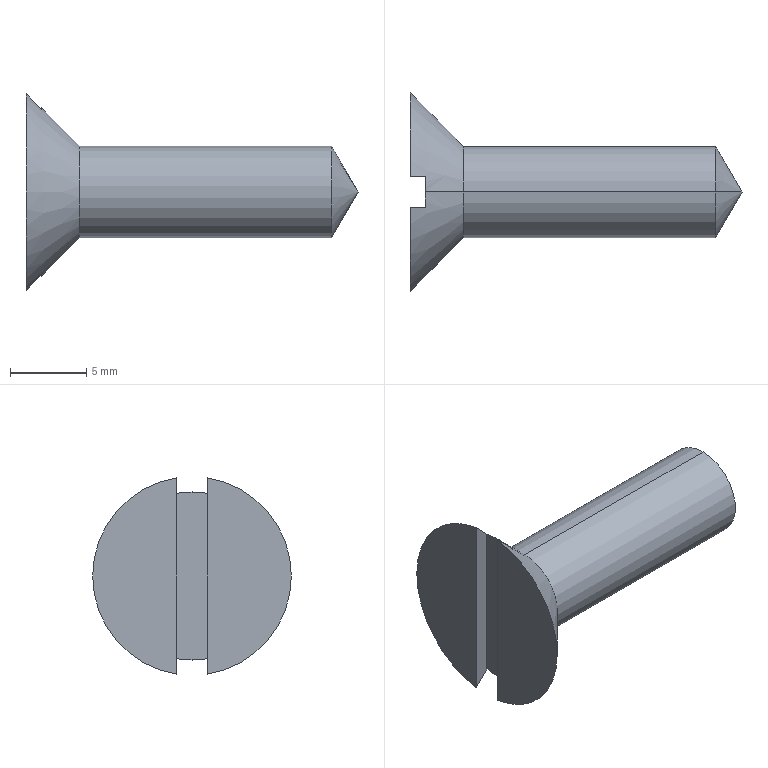Part | SolidWorks | features ICE 1, Revolution 1 | 1 solid | 11 faces | box 21.732 x 13 x 12.845 mm | volume 718.275 mm3 | plane 5 | cone 4 | cylinder 2 | commonest cylinder face diameters 6 x2